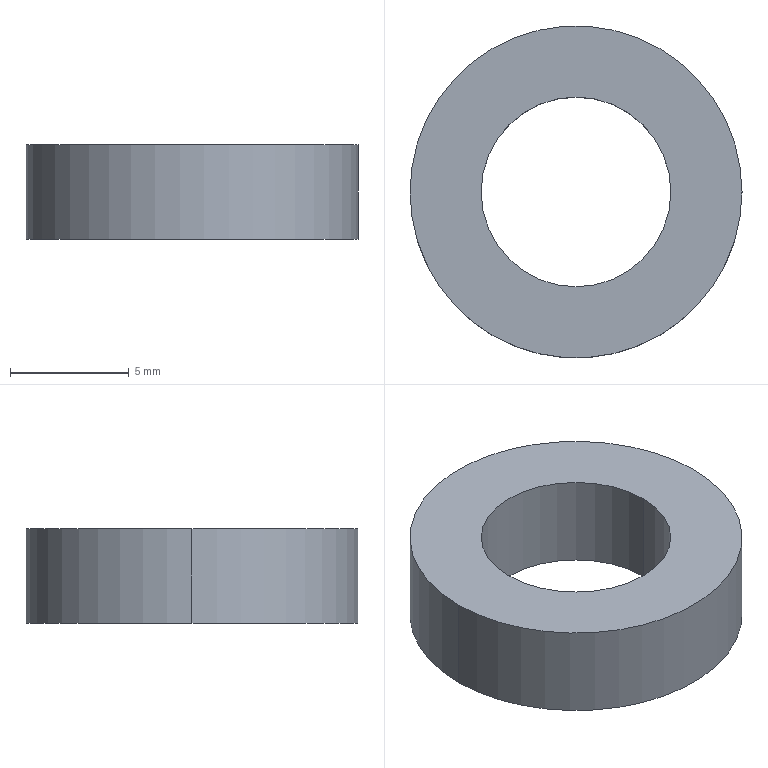Part | SolidWorks | features Extrusion 1 | 1 solid | 6 faces | box 14 x 14 x 4 mm | volume 414.69 mm3 | cylinder 4 | plane 2 | commonest cylinder face diameters 8 x2 14 x2
STEP:
#1=CARTESIAN_POINT('',(-4.,0.,4.));
#2=VERTEX_POINT('',#1);
#3=CARTESIAN_POINT('',(4.,0.,4.));
#4=VERTEX_POINT('',#3);
#5=CARTESIAN_POINT('',(0.,0.,4.));
#6=DIRECTION('',(0.,0.,1.));
#7=DIRECTION('',(1.,0.,0.));
#8=AXIS2_PLACEMENT_3D('',#5,#6,#7);
#9=CIRCLE('',#8,4.);
#10=EDGE_CURVE('',#2,#4,#9,.T.);
#11=ORIENTED_EDGE('',*,*,#10,.T.);
#12=CARTESIAN_POINT('',(4.,0.,0.));
#13=VERTEX_POINT('',#12);
#14=CARTESIAN_POINT('',(4.,0.,4.));
#15=DIRECTION('',(0.,0.,-1.));
#16=VECTOR('',#15,1000.);
#17=LINE('',#14,#16);
#18=EDGE_CURVE('',#4,#13,#17,.T.);
#19=ORIENTED_EDGE('',*,*,#18,.T.);
#20=CARTESIAN_POINT('',(-4.,0.,0.));
#21=VERTEX_POINT('',#20);
#22=CARTESIAN_POINT('',(0.,0.,0.));
#23=DIRECTION('',(0.,0.,1.));
#24=DIRECTION('',(1.,0.,0.));
#25=AXIS2_PLACEMENT_3D('',#22,#23,#24);
#26=CIRCLE('',#25,4.);
#27=EDGE_CURVE('',#21,#13,#26,.T.);
#28=ORIENTED_EDGE('',*,*,#27,.F.);
#29=CARTESIAN_POINT('',(-4.,0.,4.));
#30=DIRECTION('',(0.,0.,-1.));
#31=VECTOR('',#30,1000.);
#32=LINE('',#29,#31);
#33=EDGE_CURVE('',#2,#21,#32,.T.);
#34=ORIENTED_EDGE('',*,*,#33,.F.);
#35=EDGE_LOOP('',(#11,#19,#28,#34));
#36=FACE_OUTER_BOUND('',#35,.T.);
#37=CARTESIAN_POINT('',(0.,0.,4.));
#38=DIRECTION('',(0.,0.,-1.));
#39=DIRECTION('',(-1.,0.,0.));
#40=AXIS2_PLACEMENT_3D('',#37,#38,#39);
#41=CYLINDRICAL_SURFACE('',#40,4.);
#42=ADVANCED_FACE('',(#36),#41,.F.);
#43=CARTESIAN_POINT('',(7.,0.,4.));
#44=VERTEX_POINT('',#43);
#45=CARTESIAN_POINT('',(-7.,0.,4.));
#46=VERTEX_POINT('',#45);
#47=CARTESIAN_POINT('',(0.,0.,4.));
#48=DIRECTION('',(0.,0.,1.));
#49=DIRECTION('',(1.,0.,0.));
#50=AXIS2_PLACEMENT_3D('',#47,#48,#49);
#51=CIRCLE('',#50,7.);
#52=EDGE_CURVE('',#44,#46,#51,.T.);
#53=ORIENTED_EDGE('',*,*,#52,.F.);
#54=CARTESIAN_POINT('',(7.,0.,0.));
#55=VERTEX_POINT('',#54);
#56=CARTESIAN_POINT('',(7.,0.,4.));
#57=DIRECTION('',(0.,0.,-1.));
#58=VECTOR('',#57,1000.);
#59=LINE('',#56,#58);
#60=EDGE_CURVE('',#44,#55,#59,.T.);
#61=ORIENTED_EDGE('',*,*,#60,.T.);
#62=CARTESIAN_POINT('',(-7.,0.,0.));
#63=VERTEX_POINT('',#62);
#64=CARTESIAN_POINT('',(0.,0.,0.));
#65=DIRECTION('',(0.,0.,1.));
#66=DIRECTION('',(1.,0.,0.));
#67=AXIS2_PLACEMENT_3D('',#64,#65,#66);
#68=CIRCLE('',#67,7.);
#69=EDGE_CURVE('',#55,#63,#68,.T.);
#70=ORIENTED_EDGE('',*,*,#69,.T.);
#71=CARTESIAN_POINT('',(-7.,0.,4.));
#72=DIRECTION('',(0.,0.,-1.));
#73=VECTOR('',#72,1000.);
#74=LINE('',#71,#73);
#75=EDGE_CURVE('',#46,#63,#74,.T.);
#76=ORIENTED_EDGE('',*,*,#75,.F.);
#77=EDGE_LOOP('',(#53,#61,#70,#76));
#78=FACE_OUTER_BOUND('',#77,.T.);
#79=CARTESIAN_POINT('',(0.,0.,4.));
#80=DIRECTION('',(0.,0.,-1.));
#81=DIRECTION('',(-1.,0.,0.));
#82=AXIS2_PLACEMENT_3D('',#79,#80,#81);
#83=CYLINDRICAL_SURFACE('',#82,7.);
#84=ADVANCED_FACE('',(#78),#83,.T.);
#85=CARTESIAN_POINT('',(0.,0.,4.));
#86=DIRECTION('',(0.,0.,1.));
#87=DIRECTION('',(1.,0.,0.));
#88=AXIS2_PLACEMENT_3D('',#85,#86,#87);
#89=CIRCLE('',#88,7.);
#90=EDGE_CURVE('',#46,#44,#89,.T.);
#91=ORIENTED_EDGE('',*,*,#90,.T.);
#92=ORIENTED_EDGE('',*,*,#52,.T.);
#93=EDGE_LOOP('',(#91,#92));
#94=FACE_OUTER_BOUND('',#93,.T.);
#95=ORIENTED_EDGE('',*,*,#10,.F.);
#96=CARTESIAN_POINT('',(0.,0.,4.));
#97=DIRECTION('',(0.,0.,1.));
#98=DIRECTION('',(1.,0.,0.));
#99=AXIS2_PLACEMENT_3D('',#96,#97,#98);
#100=CIRCLE('',#99,4.);
#101=EDGE_CURVE('',#4,#2,#100,.T.);
#102=ORIENTED_EDGE('',*,*,#101,.F.);
#103=EDGE_LOOP('',(#95,#102));
#104=FACE_BOUND('',#103,.T.);
#105=CARTESIAN_POINT('',(0.,0.,4.));
#106=DIRECTION('',(0.,0.,1.));
#107=DIRECTION('',(1.,0.,0.));
#108=AXIS2_PLACEMENT_3D('',#105,#106,#107);
#109=PLANE('',#108);
#110=ADVANCED_FACE('',(#94,#104),#109,.T.);
#111=CARTESIAN_POINT('',(0.,0.,0.));
#112=DIRECTION('',(0.,0.,1.));
#113=DIRECTION('',(1.,0.,0.));
#114=AXIS2_PLACEMENT_3D('',#111,#112,#113);
#115=CIRCLE('',#114,7.);
#116=EDGE_CURVE('',#63,#55,#115,.T.);
#117=ORIENTED_EDGE('',*,*,#116,.F.);
#118=ORIENTED_EDGE('',*,*,#69,.F.);
#119=EDGE_LOOP('',(#117,#118));
#120=FACE_OUTER_BOUND('',#119,.T.);
#121=ORIENTED_EDGE('',*,*,#27,.T.);
#122=CARTESIAN_POINT('',(0.,0.,0.));
#123=DIRECTION('',(0.,0.,1.));
#124=DIRECTION('',(1.,0.,0.));
#125=AXIS2_PLACEMENT_3D('',#122,#123,#124);
#126=CIRCLE('',#125,4.);
#127=EDGE_CURVE('',#13,#21,#126,.T.);
#128=ORIENTED_EDGE('',*,*,#127,.T.);
#129=EDGE_LOOP('',(#121,#128));
#130=FACE_BOUND('',#129,.T.);
#131=CARTESIAN_POINT('',(0.,0.,0.));
#132=DIRECTION('',(0.,0.,1.));
#133=DIRECTION('',(1.,0.,0.));
#134=AXIS2_PLACEMENT_3D('',#131,#132,#133);
#135=PLANE('',#134);
#136=ADVANCED_FACE('',(#120,#130),#135,.F.);
#137=ORIENTED_EDGE('',*,*,#60,.F.);
#138=ORIENTED_EDGE('',*,*,#90,.F.);
#139=ORIENTED_EDGE('',*,*,#75,.T.);
#140=ORIENTED_EDGE('',*,*,#116,.T.);
#141=EDGE_LOOP('',(#137,#138,#139,#140));
#142=FACE_OUTER_BOUND('',#141,.T.);
#143=CARTESIAN_POINT('',(0.,0.,4.));
#144=DIRECTION('',(0.,0.,-1.));
#145=DIRECTION('',(-1.,0.,0.));
#146=AXIS2_PLACEMENT_3D('',#143,#144,#145);
#147=CYLINDRICAL_SURFACE('',#146,7.);
#148=ADVANCED_FACE('',(#142),#147,.T.);
#149=ORIENTED_EDGE('',*,*,#18,.F.);
#150=ORIENTED_EDGE('',*,*,#101,.T.);
#151=ORIENTED_EDGE('',*,*,#33,.T.);
#152=ORIENTED_EDGE('',*,*,#127,.F.);
#153=EDGE_LOOP('',(#149,#150,#151,#152));
#154=FACE_OUTER_BOUND('',#153,.T.);
#155=CARTESIAN_POINT('',(0.,0.,4.));
#156=DIRECTION('',(0.,0.,-1.));
#157=DIRECTION('',(-1.,0.,0.));
#158=AXIS2_PLACEMENT_3D('',#155,#156,#157);
#159=CYLINDRICAL_SURFACE('',#158,4.);
#160=ADVANCED_FACE('',(#154),#159,.F.);
#161=CLOSED_SHELL('',(#42,#84,#110,#136,#148,#160));
#162=MANIFOLD_SOLID_BREP('',#161);
#163=CARTESIAN_POINT('',(0.,0.,0.));
#164=DIRECTION('',(0.,0.,1.));
#165=DIRECTION('',(1.,0.,0.));
#166=AXIS2_PLACEMENT_3D('',#163,#164,#165);
#167=(LENGTH_UNIT()NAMED_UNIT(*)SI_UNIT(.MILLI.,.METRE.));
#168=UNCERTAINTY_MEASURE_WITH_UNIT(LENGTH_MEASURE(0.00001),#167,'','');
#169=(NAMED_UNIT(*)PLANE_ANGLE_UNIT()SI_UNIT($,.RADIAN.));
#170=(NAMED_UNIT(*)SI_UNIT($,.STERADIAN.)SOLID_ANGLE_UNIT());
#171=(GEOMETRIC_REPRESENTATION_CONTEXT(3)GLOBAL_UNCERTAINTY_ASSIGNED_CONTEXT((#168))GLOBAL_UNIT_ASSIGNED_CONTEXT((#167,#169,#170))REPRESENTATION_CONTEXT('',''));
#172=ADVANCED_BREP_SHAPE_REPRESENTATION('',(#162,#166),#171);